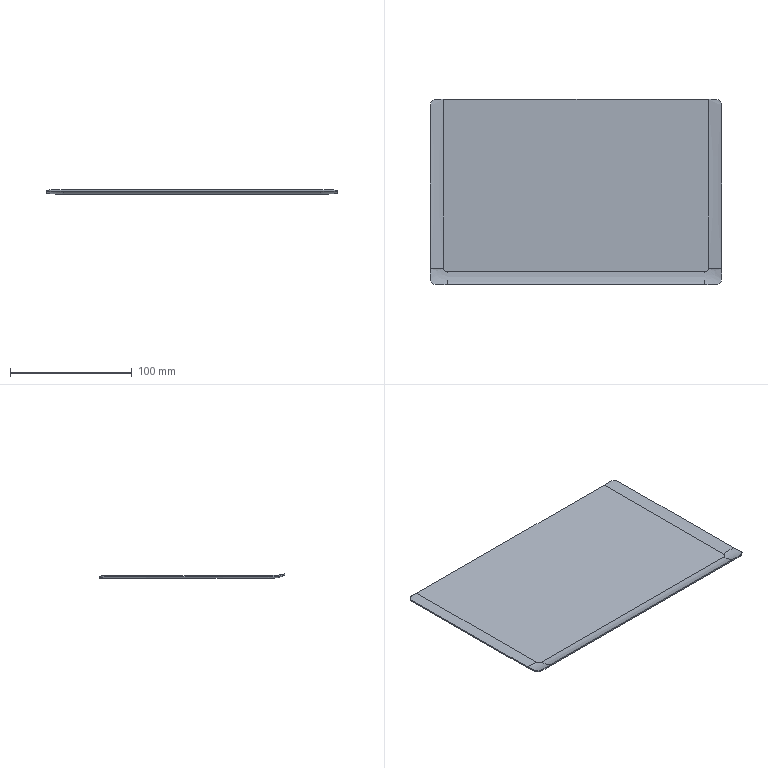Part | Creo | 1 solid | 20 faces | box 239.13 x 152.07 x 3.674 mm | volume 36465 mm3 | plane 6 | other 6 | spline 4 | cylinder 4 | commonest cylinder face diameters 10.2 x4